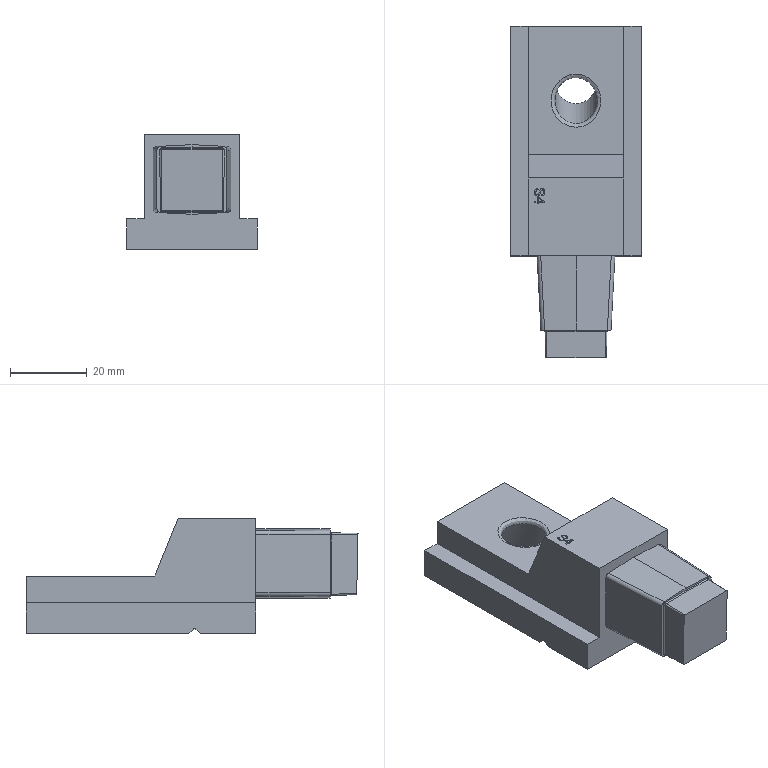Part | STEP file | lll_id38_x_t | 1 solid | 87 faces | box 34 x 86.656 x 30 mm | volume 42409 mm3 | plane 49 | other 17 | cylinder 16 | spline 5 | commonest cylinder face diameters 0.602 x10 2 x4 1 x1 11 x1